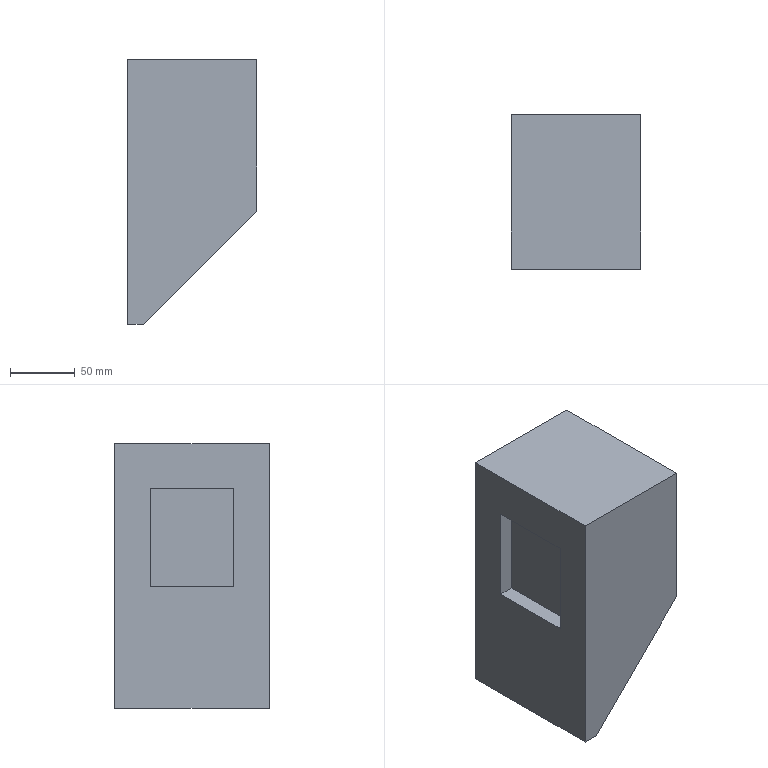Part | NX | features solid 2 | 1 solid | 12 faces | box 100 x 120 x 205 mm | volume 1939464 mm3 | plane 12
STEP:
#1=CARTESIAN_POINT('',(-978.,68.,-35.));
#2=VERTEX_POINT('',#1);
#3=CARTESIAN_POINT('',(-978.,68.,-152.321));
#4=VERTEX_POINT('',#3);
#5=CARTESIAN_POINT('',(-978.,68.,-35.));
#6=CARTESIAN_POINT('',(-978.,68.,-74.107));
#7=CARTESIAN_POINT('',(-978.,68.,-113.214));
#8=CARTESIAN_POINT('',(-978.,68.,-152.321));
#9=B_SPLINE_CURVE_WITH_KNOTS('',3,(#5,#6,#7,#8),.UNSPECIFIED.,.F.,.F.,(4,4),(0.,1.),.UNSPECIFIED.);
#10=EDGE_CURVE('',#2,#4,#9,.T.);
#11=ORIENTED_EDGE('',*,*,#10,.T.);
#12=CARTESIAN_POINT('',(-1065.679,68.,-240.));
#13=VERTEX_POINT('',#12);
#14=CARTESIAN_POINT('',(-978.,68.,-152.321));
#15=CARTESIAN_POINT('',(-1007.226,68.,-181.547));
#16=CARTESIAN_POINT('',(-1036.453,68.,-210.774));
#17=CARTESIAN_POINT('',(-1065.679,68.,-240.));
#18=B_SPLINE_CURVE_WITH_KNOTS('',3,(#14,#15,#16,#17),.UNSPECIFIED.,.F.,.F.,(4,4),(0.,1.),.UNSPECIFIED.);
#19=EDGE_CURVE('',#4,#13,#18,.T.);
#20=ORIENTED_EDGE('',*,*,#19,.T.);
#21=CARTESIAN_POINT('',(-1078.,68.,-240.));
#22=VERTEX_POINT('',#21);
#23=CARTESIAN_POINT('',(-1065.679,68.,-240.));
#24=CARTESIAN_POINT('',(-1069.786,68.,-240.));
#25=CARTESIAN_POINT('',(-1073.893,68.,-240.));
#26=CARTESIAN_POINT('',(-1078.,68.,-240.));
#27=B_SPLINE_CURVE_WITH_KNOTS('',3,(#23,#24,#25,#26),.UNSPECIFIED.,.F.,.F.,(4,4),(0.,1.),.UNSPECIFIED.);
#28=EDGE_CURVE('',#13,#22,#27,.T.);
#29=ORIENTED_EDGE('',*,*,#28,.T.);
#30=CARTESIAN_POINT('',(-1078.,68.,-35.));
#31=VERTEX_POINT('',#30);
#32=CARTESIAN_POINT('',(-1078.,68.,-240.));
#33=CARTESIAN_POINT('',(-1078.,68.,-171.667));
#34=CARTESIAN_POINT('',(-1078.,68.,-103.333));
#35=CARTESIAN_POINT('',(-1078.,68.,-35.));
#36=B_SPLINE_CURVE_WITH_KNOTS('',3,(#32,#33,#34,#35),.UNSPECIFIED.,.F.,.F.,(4,4),(0.,1.),.UNSPECIFIED.);
#37=EDGE_CURVE('',#22,#31,#36,.T.);
#38=ORIENTED_EDGE('',*,*,#37,.T.);
#39=CARTESIAN_POINT('',(-1078.,68.,-35.));
#40=CARTESIAN_POINT('',(-1044.667,68.,-35.));
#41=CARTESIAN_POINT('',(-1011.333,68.,-35.));
#42=CARTESIAN_POINT('',(-978.,68.,-35.));
#43=B_SPLINE_CURVE_WITH_KNOTS('',3,(#39,#40,#41,#42),.UNSPECIFIED.,.F.,.F.,(4,4),(0.,1.),.UNSPECIFIED.);
#44=EDGE_CURVE('',#31,#2,#43,.T.);
#45=ORIENTED_EDGE('',*,*,#44,.T.);
#46=EDGE_LOOP('',(#11,#20,#29,#38,#45));
#47=FACE_BOUND('',#46,.T.);
#48=CARTESIAN_POINT('',(-1028.,68.,-137.5));
#49=DIRECTION('',(0.,1.,0.));
#50=DIRECTION('',(-1.,0.,0.));
#51=AXIS2_PLACEMENT_3D('',#48,#49,#50);
#52=PLANE('',#51);
#53=ADVANCED_FACE('',(#47),#52,.T.);
#54=ORIENTED_EDGE('',*,*,#19,.F.);
#55=CARTESIAN_POINT('',(-978.,-52.,-152.321));
#56=VERTEX_POINT('',#55);
#57=CARTESIAN_POINT('',(-978.,68.,-152.321));
#58=CARTESIAN_POINT('',(-978.,28.,-152.321));
#59=CARTESIAN_POINT('',(-978.,-12.,-152.321));
#60=CARTESIAN_POINT('',(-978.,-52.,-152.321));
#61=B_SPLINE_CURVE_WITH_KNOTS('',3,(#57,#58,#59,#60),.UNSPECIFIED.,.F.,.F.,(4,4),(0.,1.),.UNSPECIFIED.);
#62=EDGE_CURVE('',#4,#56,#61,.T.);
#63=ORIENTED_EDGE('',*,*,#62,.T.);
#64=CARTESIAN_POINT('',(-1065.679,-52.,-240.));
#65=VERTEX_POINT('',#64);
#66=CARTESIAN_POINT('',(-978.,-52.,-152.321));
#67=CARTESIAN_POINT('',(-1007.226,-52.,-181.547));
#68=CARTESIAN_POINT('',(-1036.453,-52.,-210.774));
#69=CARTESIAN_POINT('',(-1065.679,-52.,-240.));
#70=B_SPLINE_CURVE_WITH_KNOTS('',3,(#66,#67,#68,#69),.UNSPECIFIED.,.F.,.F.,(4,4),(0.,1.),.UNSPECIFIED.);
#71=EDGE_CURVE('',#56,#65,#70,.T.);
#72=ORIENTED_EDGE('',*,*,#71,.T.);
#73=CARTESIAN_POINT('',(-1065.679,-52.,-240.));
#74=CARTESIAN_POINT('',(-1065.679,-12.,-240.));
#75=CARTESIAN_POINT('',(-1065.679,28.,-240.));
#76=CARTESIAN_POINT('',(-1065.679,68.,-240.));
#77=B_SPLINE_CURVE_WITH_KNOTS('',3,(#73,#74,#75,#76),.UNSPECIFIED.,.F.,.F.,(4,4),(0.,1.),.UNSPECIFIED.);
#78=EDGE_CURVE('',#65,#13,#77,.T.);
#79=ORIENTED_EDGE('',*,*,#78,.T.);
#80=EDGE_LOOP('',(#54,#63,#72,#79));
#81=FACE_BOUND('',#80,.T.);
#82=CARTESIAN_POINT('',(-1021.84,8.,-196.161));
#83=DIRECTION('',(0.7071,0.,-0.7071));
#84=DIRECTION('',(0.7071,0.,0.7071));
#85=AXIS2_PLACEMENT_3D('',#82,#83,#84);
#86=PLANE('',#85);
#87=ADVANCED_FACE('',(#81),#86,.T.);
#88=ORIENTED_EDGE('',*,*,#10,.F.);
#89=CARTESIAN_POINT('',(-978.,-52.,-35.));
#90=VERTEX_POINT('',#89);
#91=CARTESIAN_POINT('',(-978.,68.,-35.));
#92=CARTESIAN_POINT('',(-978.,28.,-35.));
#93=CARTESIAN_POINT('',(-978.,-12.,-35.));
#94=CARTESIAN_POINT('',(-978.,-52.,-35.));
#95=B_SPLINE_CURVE_WITH_KNOTS('',3,(#91,#92,#93,#94),.UNSPECIFIED.,.F.,.F.,(4,4),(0.,1.),.UNSPECIFIED.);
#96=EDGE_CURVE('',#2,#90,#95,.T.);
#97=ORIENTED_EDGE('',*,*,#96,.T.);
#98=CARTESIAN_POINT('',(-978.,-52.,-35.));
#99=CARTESIAN_POINT('',(-978.,-52.,-74.107));
#100=CARTESIAN_POINT('',(-978.,-52.,-113.214));
#101=CARTESIAN_POINT('',(-978.,-52.,-152.321));
#102=B_SPLINE_CURVE_WITH_KNOTS('',3,(#98,#99,#100,#101),.UNSPECIFIED.,.F.,.F.,(4,4),(0.,1.),.UNSPECIFIED.);
#103=EDGE_CURVE('',#90,#56,#102,.T.);
#104=ORIENTED_EDGE('',*,*,#103,.T.);
#105=ORIENTED_EDGE('',*,*,#62,.F.);
#106=EDGE_LOOP('',(#88,#97,#104,#105));
#107=FACE_BOUND('',#106,.T.);
#108=CARTESIAN_POINT('',(-978.,8.,-93.66));
#109=DIRECTION('',(1.,0.,0.));
#110=DIRECTION('',(0.,1.,0.));
#111=AXIS2_PLACEMENT_3D('',#108,#109,#110);
#112=PLANE('',#111);
#113=ADVANCED_FACE('',(#107),#112,.T.);
#114=ORIENTED_EDGE('',*,*,#44,.F.);
#115=CARTESIAN_POINT('',(-1078.,-52.,-35.));
#116=VERTEX_POINT('',#115);
#117=CARTESIAN_POINT('',(-1078.,68.,-35.));
#118=CARTESIAN_POINT('',(-1078.,28.,-35.));
#119=CARTESIAN_POINT('',(-1078.,-12.,-35.));
#120=CARTESIAN_POINT('',(-1078.,-52.,-35.));
#121=B_SPLINE_CURVE_WITH_KNOTS('',3,(#117,#118,#119,#120),.UNSPECIFIED.,.F.,.F.,(4,4),(0.,1.),.UNSPECIFIED.);
#122=EDGE_CURVE('',#31,#116,#121,.T.);
#123=ORIENTED_EDGE('',*,*,#122,.T.);
#124=CARTESIAN_POINT('',(-1078.,-52.,-35.));
#125=CARTESIAN_POINT('',(-1044.667,-52.,-35.));
#126=CARTESIAN_POINT('',(-1011.333,-52.,-35.));
#127=CARTESIAN_POINT('',(-978.,-52.,-35.));
#128=B_SPLINE_CURVE_WITH_KNOTS('',3,(#124,#125,#126,#127),.UNSPECIFIED.,.F.,.F.,(4,4),(0.,1.),.UNSPECIFIED.);
#129=EDGE_CURVE('',#116,#90,#128,.T.);
#130=ORIENTED_EDGE('',*,*,#129,.T.);
#131=ORIENTED_EDGE('',*,*,#96,.F.);
#132=EDGE_LOOP('',(#114,#123,#130,#131));
#133=FACE_BOUND('',#132,.T.);
#134=CARTESIAN_POINT('',(-1028.,8.,-35.));
#135=DIRECTION('',(0.,0.,1.));
#136=DIRECTION('',(0.,-1.,0.));
#137=AXIS2_PLACEMENT_3D('',#134,#135,#136);
#138=PLANE('',#137);
#139=ADVANCED_FACE('',(#133),#138,.T.);
#140=CARTESIAN_POINT('',(-1078.,40.5,-70.));
#141=VERTEX_POINT('',#140);
#142=CARTESIAN_POINT('',(-1078.,-24.5,-70.));
#143=VERTEX_POINT('',#142);
#144=CARTESIAN_POINT('',(-1078.,40.5,-70.));
#145=CARTESIAN_POINT('',(-1078.,18.833,-70.));
#146=CARTESIAN_POINT('',(-1078.,-2.833,-70.));
#147=CARTESIAN_POINT('',(-1078.,-24.5,-70.));
#148=B_SPLINE_CURVE_WITH_KNOTS('',3,(#144,#145,#146,#147),.UNSPECIFIED.,.F.,.F.,(4,4),(0.,1.),.UNSPECIFIED.);
#149=EDGE_CURVE('',#141,#143,#148,.T.);
#150=ORIENTED_EDGE('',*,*,#149,.T.);
#151=CARTESIAN_POINT('',(-1078.,-24.5,-146.));
#152=VERTEX_POINT('',#151);
#153=CARTESIAN_POINT('',(-1078.,-24.5,-70.));
#154=CARTESIAN_POINT('',(-1078.,-24.5,-95.333));
#155=CARTESIAN_POINT('',(-1078.,-24.5,-120.667));
#156=CARTESIAN_POINT('',(-1078.,-24.5,-146.));
#157=B_SPLINE_CURVE_WITH_KNOTS('',3,(#153,#154,#155,#156),.UNSPECIFIED.,.F.,.F.,(4,4),(0.,1.),.UNSPECIFIED.);
#158=EDGE_CURVE('',#143,#152,#157,.T.);
#159=ORIENTED_EDGE('',*,*,#158,.T.);
#160=CARTESIAN_POINT('',(-1078.,40.5,-146.));
#161=VERTEX_POINT('',#160);
#162=CARTESIAN_POINT('',(-1078.,-24.5,-146.));
#163=CARTESIAN_POINT('',(-1078.,-2.833,-146.));
#164=CARTESIAN_POINT('',(-1078.,18.833,-146.));
#165=CARTESIAN_POINT('',(-1078.,40.5,-146.));
#166=B_SPLINE_CURVE_WITH_KNOTS('',3,(#162,#163,#164,#165),.UNSPECIFIED.,.F.,.F.,(4,4),(0.,1.),.UNSPECIFIED.);
#167=EDGE_CURVE('',#152,#161,#166,.T.);
#168=ORIENTED_EDGE('',*,*,#167,.T.);
#169=CARTESIAN_POINT('',(-1078.,40.5,-146.));
#170=CARTESIAN_POINT('',(-1078.,40.5,-120.667));
#171=CARTESIAN_POINT('',(-1078.,40.5,-95.333));
#172=CARTESIAN_POINT('',(-1078.,40.5,-70.));
#173=B_SPLINE_CURVE_WITH_KNOTS('',3,(#169,#170,#171,#172),.UNSPECIFIED.,.F.,.F.,(4,4),(0.,1.),.UNSPECIFIED.);
#174=EDGE_CURVE('',#161,#141,#173,.T.);
#175=ORIENTED_EDGE('',*,*,#174,.T.);
#176=EDGE_LOOP('',(#150,#159,#168,#175));
#177=FACE_BOUND('',#176,.T.);
#178=ORIENTED_EDGE('',*,*,#37,.F.);
#179=CARTESIAN_POINT('',(-1078.,-52.,-240.));
#180=VERTEX_POINT('',#179);
#181=CARTESIAN_POINT('',(-1078.,68.,-240.));
#182=CARTESIAN_POINT('',(-1078.,28.,-240.));
#183=CARTESIAN_POINT('',(-1078.,-12.,-240.));
#184=CARTESIAN_POINT('',(-1078.,-52.,-240.));
#185=B_SPLINE_CURVE_WITH_KNOTS('',3,(#181,#182,#183,#184),.UNSPECIFIED.,.F.,.F.,(4,4),(0.,1.),.UNSPECIFIED.);
#186=EDGE_CURVE('',#22,#180,#185,.T.);
#187=ORIENTED_EDGE('',*,*,#186,.T.);
#188=CARTESIAN_POINT('',(-1078.,-52.,-240.));
#189=CARTESIAN_POINT('',(-1078.,-52.,-171.667));
#190=CARTESIAN_POINT('',(-1078.,-52.,-103.333));
#191=CARTESIAN_POINT('',(-1078.,-52.,-35.));
#192=B_SPLINE_CURVE_WITH_KNOTS('',3,(#188,#189,#190,#191),.UNSPECIFIED.,.F.,.F.,(4,4),(0.,1.),.UNSPECIFIED.);
#193=EDGE_CURVE('',#180,#116,#192,.T.);
#194=ORIENTED_EDGE('',*,*,#193,.T.);
#195=ORIENTED_EDGE('',*,*,#122,.F.);
#196=EDGE_LOOP('',(#178,#187,#194,#195));
#197=FACE_BOUND('',#196,.T.);
#198=CARTESIAN_POINT('',(-1078.,8.,-137.5));
#199=DIRECTION('',(-1.,0.,0.));
#200=DIRECTION('',(0.,-1.,0.));
#201=AXIS2_PLACEMENT_3D('',#198,#199,#200);
#202=PLANE('',#201);
#203=ADVANCED_FACE('',(#177,#197),#202,.T.);
#204=ORIENTED_EDGE('',*,*,#28,.F.);
#205=ORIENTED_EDGE('',*,*,#78,.F.);
#206=CARTESIAN_POINT('',(-1065.679,-52.,-240.));
#207=CARTESIAN_POINT('',(-1069.786,-52.,-240.));
#208=CARTESIAN_POINT('',(-1073.893,-52.,-240.));
#209=CARTESIAN_POINT('',(-1078.,-52.,-240.));
#210=B_SPLINE_CURVE_WITH_KNOTS('',3,(#206,#207,#208,#209),.UNSPECIFIED.,.F.,.F.,(4,4),(0.,1.),.UNSPECIFIED.);
#211=EDGE_CURVE('',#65,#180,#210,.T.);
#212=ORIENTED_EDGE('',*,*,#211,.T.);
#213=ORIENTED_EDGE('',*,*,#186,.F.);
#214=EDGE_LOOP('',(#204,#205,#212,#213));
#215=FACE_BOUND('',#214,.T.);
#216=CARTESIAN_POINT('',(-1071.84,8.,-240.));
#217=DIRECTION('',(0.,0.,-1.));
#218=DIRECTION('',(0.,1.,0.));
#219=AXIS2_PLACEMENT_3D('',#216,#217,#218);
#220=PLANE('',#219);
#221=ADVANCED_FACE('',(#215),#220,.T.);
#222=ORIENTED_EDGE('',*,*,#71,.F.);
#223=ORIENTED_EDGE('',*,*,#103,.F.);
#224=ORIENTED_EDGE('',*,*,#129,.F.);
#225=ORIENTED_EDGE('',*,*,#193,.F.);
#226=ORIENTED_EDGE('',*,*,#211,.F.);
#227=EDGE_LOOP('',(#222,#223,#224,#225,#226));
#228=FACE_BOUND('',#227,.T.);
#229=CARTESIAN_POINT('',(-1028.,-52.,-137.5));
#230=DIRECTION('',(0.,-1.,0.));
#231=DIRECTION('',(1.,0.,0.));
#232=AXIS2_PLACEMENT_3D('',#229,#230,#231);
#233=PLANE('',#232);
#234=ADVANCED_FACE('',(#228),#233,.T.);
#235=CARTESIAN_POINT('',(-1066.,-24.5,-146.));
#236=VERTEX_POINT('',#235);
#237=CARTESIAN_POINT('',(-1066.,-24.5,-146.));
#238=CARTESIAN_POINT('',(-1070.,-24.5,-146.));
#239=CARTESIAN_POINT('',(-1074.,-24.5,-146.));
#240=CARTESIAN_POINT('',(-1078.,-24.5,-146.));
#241=B_SPLINE_CURVE_WITH_KNOTS('',3,(#237,#238,#239,#240),.UNSPECIFIED.,.F.,.F.,(4,4),(0.,1.),.UNSPECIFIED.);
#242=EDGE_CURVE('',#236,#152,#241,.T.);
#243=ORIENTED_EDGE('',*,*,#242,.T.);
#244=ORIENTED_EDGE('',*,*,#158,.F.);
#245=CARTESIAN_POINT('',(-1066.,-24.5,-70.));
#246=VERTEX_POINT('',#245);
#247=CARTESIAN_POINT('',(-1078.,-24.5,-70.));
#248=CARTESIAN_POINT('',(-1074.,-24.5,-70.));
#249=CARTESIAN_POINT('',(-1070.,-24.5,-70.));
#250=CARTESIAN_POINT('',(-1066.,-24.5,-70.));
#251=B_SPLINE_CURVE_WITH_KNOTS('',3,(#247,#248,#249,#250),.UNSPECIFIED.,.F.,.F.,(4,4),(0.,1.),.UNSPECIFIED.);
#252=EDGE_CURVE('',#143,#246,#251,.T.);
#253=ORIENTED_EDGE('',*,*,#252,.T.);
#254=CARTESIAN_POINT('',(-1066.,-24.5,-70.));
#255=CARTESIAN_POINT('',(-1066.,-24.5,-95.333));
#256=CARTESIAN_POINT('',(-1066.,-24.5,-120.667));
#257=CARTESIAN_POINT('',(-1066.,-24.5,-146.));
#258=B_SPLINE_CURVE_WITH_KNOTS('',3,(#254,#255,#256,#257),.UNSPECIFIED.,.F.,.F.,(4,4),(0.,1.),.UNSPECIFIED.);
#259=EDGE_CURVE('',#246,#236,#258,.T.);
#260=ORIENTED_EDGE('',*,*,#259,.T.);
#261=EDGE_LOOP('',(#243,#244,#253,#260));
#262=FACE_BOUND('',#261,.T.);
#263=CARTESIAN_POINT('',(-1072.,-24.5,-108.));
#264=DIRECTION('',(0.,1.,0.));
#265=DIRECTION('',(-1.,0.,0.));
#266=AXIS2_PLACEMENT_3D('',#263,#264,#265);
#267=PLANE('',#266);
#268=ADVANCED_FACE('',(#262),#267,.T.);
#269=CARTESIAN_POINT('',(-1066.,40.5,-70.));
#270=VERTEX_POINT('',#269);
#271=CARTESIAN_POINT('',(-1078.,40.5,-70.));
#272=CARTESIAN_POINT('',(-1074.,40.5,-70.));
#273=CARTESIAN_POINT('',(-1070.,40.5,-70.));
#274=CARTESIAN_POINT('',(-1066.,40.5,-70.));
#275=B_SPLINE_CURVE_WITH_KNOTS('',3,(#271,#272,#273,#274),.UNSPECIFIED.,.F.,.F.,(4,4),(0.,1.),.UNSPECIFIED.);
#276=EDGE_CURVE('',#141,#270,#275,.T.);
#277=ORIENTED_EDGE('',*,*,#276,.T.);
#278=CARTESIAN_POINT('',(-1066.,40.5,-70.));
#279=CARTESIAN_POINT('',(-1066.,18.833,-70.));
#280=CARTESIAN_POINT('',(-1066.,-2.833,-70.));
#281=CARTESIAN_POINT('',(-1066.,-24.5,-70.));
#282=B_SPLINE_CURVE_WITH_KNOTS('',3,(#278,#279,#280,#281),.UNSPECIFIED.,.F.,.F.,(4,4),(0.,1.),.UNSPECIFIED.);
#283=EDGE_CURVE('',#270,#246,#282,.T.);
#284=ORIENTED_EDGE('',*,*,#283,.T.);
#285=ORIENTED_EDGE('',*,*,#252,.F.);
#286=ORIENTED_EDGE('',*,*,#149,.F.);
#287=EDGE_LOOP('',(#277,#284,#285,#286));
#288=FACE_BOUND('',#287,.T.);
#289=CARTESIAN_POINT('',(-1072.,8.,-70.));
#290=DIRECTION('',(0.,0.,-1.));
#291=DIRECTION('',(0.,1.,0.));
#292=AXIS2_PLACEMENT_3D('',#289,#290,#291);
#293=PLANE('',#292);
#294=ADVANCED_FACE('',(#288),#293,.T.);
#295=ORIENTED_EDGE('',*,*,#276,.F.);
#296=ORIENTED_EDGE('',*,*,#174,.F.);
#297=CARTESIAN_POINT('',(-1066.,40.5,-146.));
#298=VERTEX_POINT('',#297);
#299=CARTESIAN_POINT('',(-1078.,40.5,-146.));
#300=CARTESIAN_POINT('',(-1074.,40.5,-146.));
#301=CARTESIAN_POINT('',(-1070.,40.5,-146.));
#302=CARTESIAN_POINT('',(-1066.,40.5,-146.));
#303=B_SPLINE_CURVE_WITH_KNOTS('',3,(#299,#300,#301,#302),.UNSPECIFIED.,.F.,.F.,(4,4),(0.,1.),.UNSPECIFIED.);
#304=EDGE_CURVE('',#161,#298,#303,.T.);
#305=ORIENTED_EDGE('',*,*,#304,.T.);
#306=CARTESIAN_POINT('',(-1066.,40.5,-146.));
#307=CARTESIAN_POINT('',(-1066.,40.5,-120.667));
#308=CARTESIAN_POINT('',(-1066.,40.5,-95.333));
#309=CARTESIAN_POINT('',(-1066.,40.5,-70.));
#310=B_SPLINE_CURVE_WITH_KNOTS('',3,(#306,#307,#308,#309),.UNSPECIFIED.,.F.,.F.,(4,4),(0.,1.),.UNSPECIFIED.);
#311=EDGE_CURVE('',#298,#270,#310,.T.);
#312=ORIENTED_EDGE('',*,*,#311,.T.);
#313=EDGE_LOOP('',(#295,#296,#305,#312));
#314=FACE_BOUND('',#313,.T.);
#315=CARTESIAN_POINT('',(-1072.,40.5,-108.));
#316=DIRECTION('',(0.,-1.,0.));
#317=DIRECTION('',(1.,0.,0.));
#318=AXIS2_PLACEMENT_3D('',#315,#316,#317);
#319=PLANE('',#318);
#320=ADVANCED_FACE('',(#314),#319,.T.);
#321=ORIENTED_EDGE('',*,*,#304,.F.);
#322=ORIENTED_EDGE('',*,*,#167,.F.);
#323=ORIENTED_EDGE('',*,*,#242,.F.);
#324=CARTESIAN_POINT('',(-1066.,-24.5,-146.));
#325=CARTESIAN_POINT('',(-1066.,-2.833,-146.));
#326=CARTESIAN_POINT('',(-1066.,18.833,-146.));
#327=CARTESIAN_POINT('',(-1066.,40.5,-146.));
#328=B_SPLINE_CURVE_WITH_KNOTS('',3,(#324,#325,#326,#327),.UNSPECIFIED.,.F.,.F.,(4,4),(0.,1.),.UNSPECIFIED.);
#329=EDGE_CURVE('',#236,#298,#328,.T.);
#330=ORIENTED_EDGE('',*,*,#329,.T.);
#331=EDGE_LOOP('',(#321,#322,#323,#330));
#332=FACE_BOUND('',#331,.T.);
#333=CARTESIAN_POINT('',(-1072.,8.,-146.));
#334=DIRECTION('',(0.,0.,1.));
#335=DIRECTION('',(0.,-1.,0.));
#336=AXIS2_PLACEMENT_3D('',#333,#334,#335);
#337=PLANE('',#336);
#338=ADVANCED_FACE('',(#332),#337,.T.);
#339=ORIENTED_EDGE('',*,*,#311,.F.);
#340=ORIENTED_EDGE('',*,*,#329,.F.);
#341=ORIENTED_EDGE('',*,*,#259,.F.);
#342=ORIENTED_EDGE('',*,*,#283,.F.);
#343=EDGE_LOOP('',(#339,#340,#341,#342));
#344=FACE_BOUND('',#343,.T.);
#345=CARTESIAN_POINT('',(-1066.,8.,-108.));
#346=DIRECTION('',(-1.,0.,0.));
#347=DIRECTION('',(0.,-1.,0.));
#348=AXIS2_PLACEMENT_3D('',#345,#346,#347);
#349=PLANE('',#348);
#350=ADVANCED_FACE('',(#344),#349,.T.);
#351=CLOSED_SHELL('',(#53,#87,#113,#139,#203,#221,#234,#268,#294,#320,#338,#350));
#352=MANIFOLD_SOLID_BREP('',#351);
#353=(LENGTH_UNIT()NAMED_UNIT(*)SI_UNIT(.MILLI.,.METRE.));
#354=UNCERTAINTY_MEASURE_WITH_UNIT(LENGTH_MEASURE(0.0508),#353,'','');
#355=(NAMED_UNIT(*)PLANE_ANGLE_UNIT()SI_UNIT($,.RADIAN.));
#356=(NAMED_UNIT(*)SI_UNIT($,.STERADIAN.)SOLID_ANGLE_UNIT());
#357=(GEOMETRIC_REPRESENTATION_CONTEXT(3)GLOBAL_UNCERTAINTY_ASSIGNED_CONTEXT((#354))GLOBAL_UNIT_ASSIGNED_CONTEXT((#353,#355,#356))REPRESENTATION_CONTEXT('',''));
#358=ADVANCED_BREP_SHAPE_REPRESENTATION('',(#352),#357);